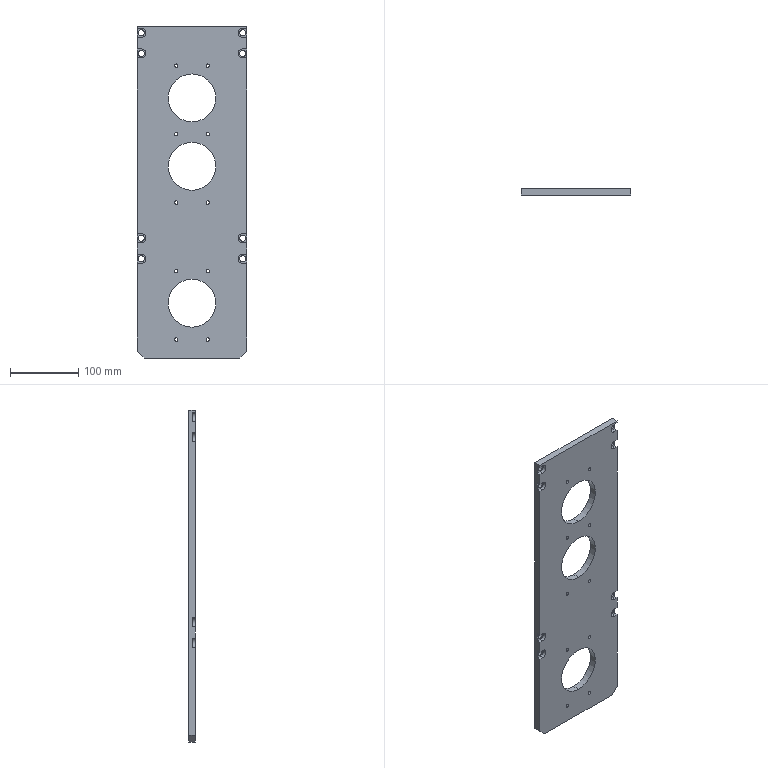Part | SolidWorks | features BaseBody 1 | 1 solid | 82 faces | box 160 x 10 x 485 mm | volume 649264 mm3 | cylinder 50 | plane 32 | commonest cylinder face diameters 5 x20 9 x16 13 x8 70 x6